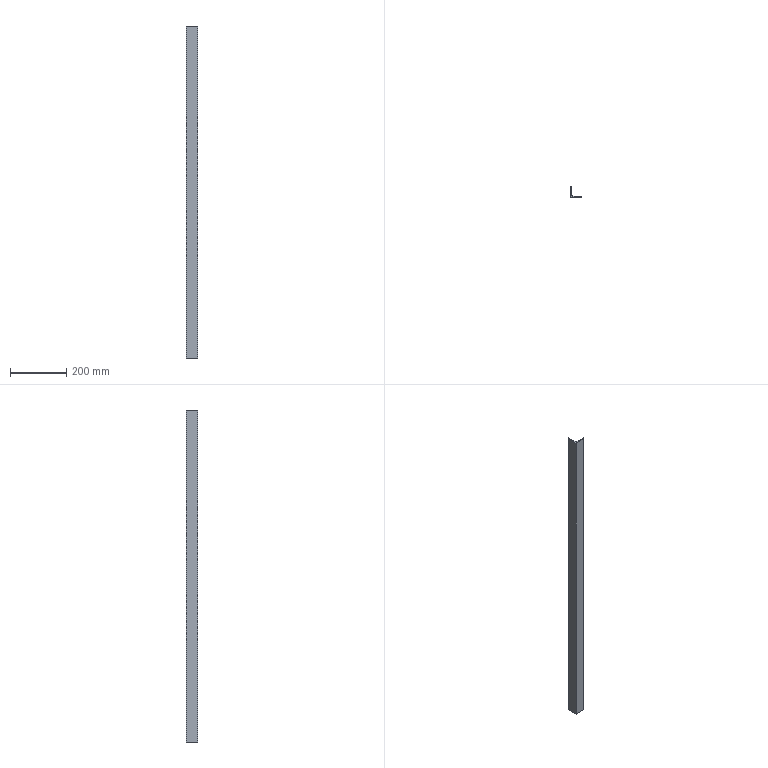Part | SolidWorks | features Extrusion 1 | 1 solid | 11 faces | box 40 x 40 x 1185 mm | volume 366598 mm3 | plane 8 | cylinder 3 | commonest cylinder face diameters 0.02 x2 10 x1
STEP:
#1=CARTESIAN_POINT('',(0.,0.,0.));
#2=VERTEX_POINT('',#1);
#3=CARTESIAN_POINT('',(40.,0.,0.));
#4=VERTEX_POINT('',#3);
#5=CARTESIAN_POINT('',(40.,0.,0.));
#6=DIRECTION('',(1.,0.,0.));
#7=VECTOR('',#6,1000.);
#8=LINE('',#5,#7);
#9=EDGE_CURVE('',#2,#4,#8,.T.);
#10=ORIENTED_EDGE('',*,*,#9,.T.);
#11=CARTESIAN_POINT('',(40.,0.,1185.));
#12=VERTEX_POINT('',#11);
#13=CARTESIAN_POINT('',(40.,0.,1185.));
#14=DIRECTION('',(0.,0.,-1.));
#15=VECTOR('',#14,1000.);
#16=LINE('',#13,#15);
#17=EDGE_CURVE('',#12,#4,#16,.T.);
#18=ORIENTED_EDGE('',*,*,#17,.F.);
#19=CARTESIAN_POINT('',(0.,0.,1185.));
#20=VERTEX_POINT('',#19);
#21=CARTESIAN_POINT('',(40.,0.,1185.));
#22=DIRECTION('',(1.,0.,0.));
#23=VECTOR('',#22,1000.);
#24=LINE('',#21,#23);
#25=EDGE_CURVE('',#20,#12,#24,.T.);
#26=ORIENTED_EDGE('',*,*,#25,.F.);
#27=CARTESIAN_POINT('',(0.,0.,1185.));
#28=DIRECTION('',(0.,0.,-1.));
#29=VECTOR('',#28,1000.);
#30=LINE('',#27,#29);
#31=EDGE_CURVE('',#20,#2,#30,.T.);
#32=ORIENTED_EDGE('',*,*,#31,.T.);
#33=EDGE_LOOP('',(#10,#18,#26,#32));
#34=FACE_OUTER_BOUND('',#33,.T.);
#35=CARTESIAN_POINT('',(40.,0.,1185.));
#36=DIRECTION('',(0.,1.,0.));
#37=DIRECTION('',(-1.,0.,0.));
#38=AXIS2_PLACEMENT_3D('',#35,#36,#37);
#39=PLANE('',#38);
#40=ADVANCED_FACE('',(#34),#39,.F.);
#41=CARTESIAN_POINT('',(40.,3.99,0.));
#42=VERTEX_POINT('',#41);
#43=CARTESIAN_POINT('',(40.,3.99,0.));
#44=DIRECTION('',(0.,1.,0.));
#45=VECTOR('',#44,1000.);
#46=LINE('',#43,#45);
#47=EDGE_CURVE('',#4,#42,#46,.T.);
#48=ORIENTED_EDGE('',*,*,#47,.T.);
#49=CARTESIAN_POINT('',(40.,3.99,1185.));
#50=VERTEX_POINT('',#49);
#51=CARTESIAN_POINT('',(40.,3.99,1185.));
#52=DIRECTION('',(0.,0.,-1.));
#53=VECTOR('',#52,1000.);
#54=LINE('',#51,#53);
#55=EDGE_CURVE('',#50,#42,#54,.T.);
#56=ORIENTED_EDGE('',*,*,#55,.F.);
#57=CARTESIAN_POINT('',(40.,3.99,1185.));
#58=DIRECTION('',(0.,1.,0.));
#59=VECTOR('',#58,1000.);
#60=LINE('',#57,#59);
#61=EDGE_CURVE('',#12,#50,#60,.T.);
#62=ORIENTED_EDGE('',*,*,#61,.F.);
#63=ORIENTED_EDGE('',*,*,#17,.T.);
#64=EDGE_LOOP('',(#48,#56,#62,#63));
#65=FACE_OUTER_BOUND('',#64,.T.);
#66=CARTESIAN_POINT('',(40.,3.99,1185.));
#67=DIRECTION('',(-1.,0.,0.));
#68=DIRECTION('',(0.,-1.,0.));
#69=AXIS2_PLACEMENT_3D('',#66,#67,#68);
#70=PLANE('',#69);
#71=ADVANCED_FACE('',(#65),#70,.F.);
#72=CARTESIAN_POINT('',(39.99,4.,0.));
#73=VERTEX_POINT('',#72);
#74=CARTESIAN_POINT('',(39.99,3.99,0.));
#75=DIRECTION('',(0.,0.,1.));
#76=DIRECTION('',(1.,0.,0.));
#77=AXIS2_PLACEMENT_3D('',#74,#75,#76);
#78=CIRCLE('',#77,0.01);
#79=EDGE_CURVE('',#42,#73,#78,.T.);
#80=ORIENTED_EDGE('',*,*,#79,.T.);
#81=CARTESIAN_POINT('',(39.99,4.,1185.));
#82=VERTEX_POINT('',#81);
#83=CARTESIAN_POINT('',(39.99,4.,1185.));
#84=DIRECTION('',(0.,0.,-1.));
#85=VECTOR('',#84,1000.);
#86=LINE('',#83,#85);
#87=EDGE_CURVE('',#82,#73,#86,.T.);
#88=ORIENTED_EDGE('',*,*,#87,.F.);
#89=CARTESIAN_POINT('',(39.99,3.99,1185.));
#90=DIRECTION('',(0.,0.,1.));
#91=DIRECTION('',(1.,0.,0.));
#92=AXIS2_PLACEMENT_3D('',#89,#90,#91);
#93=CIRCLE('',#92,0.01);
#94=EDGE_CURVE('',#50,#82,#93,.T.);
#95=ORIENTED_EDGE('',*,*,#94,.F.);
#96=ORIENTED_EDGE('',*,*,#55,.T.);
#97=EDGE_LOOP('',(#80,#88,#95,#96));
#98=FACE_OUTER_BOUND('',#97,.T.);
#99=CARTESIAN_POINT('',(39.99,3.99,1185.));
#100=DIRECTION('',(0.,0.,-1.));
#101=DIRECTION('',(-1.,0.,0.));
#102=AXIS2_PLACEMENT_3D('',#99,#100,#101);
#103=CYLINDRICAL_SURFACE('',#102,0.01);
#104=ADVANCED_FACE('',(#98),#103,.T.);
#105=CARTESIAN_POINT('',(9.,4.,0.));
#106=VERTEX_POINT('',#105);
#107=CARTESIAN_POINT('',(9.,4.,0.));
#108=DIRECTION('',(-1.,0.,0.));
#109=VECTOR('',#108,1000.);
#110=LINE('',#107,#109);
#111=EDGE_CURVE('',#73,#106,#110,.T.);
#112=ORIENTED_EDGE('',*,*,#111,.T.);
#113=CARTESIAN_POINT('',(9.,4.,1185.));
#114=VERTEX_POINT('',#113);
#115=CARTESIAN_POINT('',(9.,4.,1185.));
#116=DIRECTION('',(0.,0.,-1.));
#117=VECTOR('',#116,1000.);
#118=LINE('',#115,#117);
#119=EDGE_CURVE('',#114,#106,#118,.T.);
#120=ORIENTED_EDGE('',*,*,#119,.F.);
#121=CARTESIAN_POINT('',(9.,4.,1185.));
#122=DIRECTION('',(-1.,0.,0.));
#123=VECTOR('',#122,1000.);
#124=LINE('',#121,#123);
#125=EDGE_CURVE('',#82,#114,#124,.T.);
#126=ORIENTED_EDGE('',*,*,#125,.F.);
#127=ORIENTED_EDGE('',*,*,#87,.T.);
#128=EDGE_LOOP('',(#112,#120,#126,#127));
#129=FACE_OUTER_BOUND('',#128,.T.);
#130=CARTESIAN_POINT('',(9.,4.,1185.));
#131=DIRECTION('',(0.,-1.,0.));
#132=DIRECTION('',(1.,0.,0.));
#133=AXIS2_PLACEMENT_3D('',#130,#131,#132);
#134=PLANE('',#133);
#135=ADVANCED_FACE('',(#129),#134,.F.);
#136=CARTESIAN_POINT('',(4.,9.,0.));
#137=VERTEX_POINT('',#136);
#138=CARTESIAN_POINT('',(9.,9.,0.));
#139=DIRECTION('',(0.,0.,-1.));
#140=DIRECTION('',(-1.,0.,0.));
#141=AXIS2_PLACEMENT_3D('',#138,#139,#140);
#142=CIRCLE('',#141,5.);
#143=EDGE_CURVE('',#106,#137,#142,.T.);
#144=ORIENTED_EDGE('',*,*,#143,.T.);
#145=CARTESIAN_POINT('',(4.,9.,1185.));
#146=VERTEX_POINT('',#145);
#147=CARTESIAN_POINT('',(4.,9.,1185.));
#148=DIRECTION('',(0.,0.,-1.));
#149=VECTOR('',#148,1000.);
#150=LINE('',#147,#149);
#151=EDGE_CURVE('',#146,#137,#150,.T.);
#152=ORIENTED_EDGE('',*,*,#151,.F.);
#153=CARTESIAN_POINT('',(9.,9.,1185.));
#154=DIRECTION('',(0.,0.,-1.));
#155=DIRECTION('',(-1.,0.,0.));
#156=AXIS2_PLACEMENT_3D('',#153,#154,#155);
#157=CIRCLE('',#156,5.);
#158=EDGE_CURVE('',#114,#146,#157,.T.);
#159=ORIENTED_EDGE('',*,*,#158,.F.);
#160=ORIENTED_EDGE('',*,*,#119,.T.);
#161=EDGE_LOOP('',(#144,#152,#159,#160));
#162=FACE_OUTER_BOUND('',#161,.T.);
#163=CARTESIAN_POINT('',(9.,9.,1185.));
#164=DIRECTION('',(0.,0.,-1.));
#165=DIRECTION('',(-1.,0.,0.));
#166=AXIS2_PLACEMENT_3D('',#163,#164,#165);
#167=CYLINDRICAL_SURFACE('',#166,5.);
#168=ADVANCED_FACE('',(#162),#167,.F.);
#169=CARTESIAN_POINT('',(4.,39.99,0.));
#170=VERTEX_POINT('',#169);
#171=CARTESIAN_POINT('',(4.,39.99,0.));
#172=DIRECTION('',(0.,1.,0.));
#173=VECTOR('',#172,1000.);
#174=LINE('',#171,#173);
#175=EDGE_CURVE('',#137,#170,#174,.T.);
#176=ORIENTED_EDGE('',*,*,#175,.T.);
#177=CARTESIAN_POINT('',(4.,39.99,1185.));
#178=VERTEX_POINT('',#177);
#179=CARTESIAN_POINT('',(4.,39.99,1185.));
#180=DIRECTION('',(0.,0.,-1.));
#181=VECTOR('',#180,1000.);
#182=LINE('',#179,#181);
#183=EDGE_CURVE('',#178,#170,#182,.T.);
#184=ORIENTED_EDGE('',*,*,#183,.F.);
#185=CARTESIAN_POINT('',(4.,39.99,1185.));
#186=DIRECTION('',(0.,1.,0.));
#187=VECTOR('',#186,1000.);
#188=LINE('',#185,#187);
#189=EDGE_CURVE('',#146,#178,#188,.T.);
#190=ORIENTED_EDGE('',*,*,#189,.F.);
#191=ORIENTED_EDGE('',*,*,#151,.T.);
#192=EDGE_LOOP('',(#176,#184,#190,#191));
#193=FACE_OUTER_BOUND('',#192,.T.);
#194=CARTESIAN_POINT('',(4.,39.99,1185.));
#195=DIRECTION('',(-1.,0.,0.));
#196=DIRECTION('',(0.,-1.,0.));
#197=AXIS2_PLACEMENT_3D('',#194,#195,#196);
#198=PLANE('',#197);
#199=ADVANCED_FACE('',(#193),#198,.F.);
#200=CARTESIAN_POINT('',(3.99,40.,0.));
#201=VERTEX_POINT('',#200);
#202=CARTESIAN_POINT('',(3.99,39.99,0.));
#203=DIRECTION('',(0.,0.,1.));
#204=DIRECTION('',(1.,0.,0.));
#205=AXIS2_PLACEMENT_3D('',#202,#203,#204);
#206=CIRCLE('',#205,0.01);
#207=EDGE_CURVE('',#170,#201,#206,.T.);
#208=ORIENTED_EDGE('',*,*,#207,.T.);
#209=CARTESIAN_POINT('',(3.99,40.,1185.));
#210=VERTEX_POINT('',#209);
#211=CARTESIAN_POINT('',(3.99,40.,1185.));
#212=DIRECTION('',(0.,0.,-1.));
#213=VECTOR('',#212,1000.);
#214=LINE('',#211,#213);
#215=EDGE_CURVE('',#210,#201,#214,.T.);
#216=ORIENTED_EDGE('',*,*,#215,.F.);
#217=CARTESIAN_POINT('',(3.99,39.99,1185.));
#218=DIRECTION('',(0.,0.,1.));
#219=DIRECTION('',(1.,0.,0.));
#220=AXIS2_PLACEMENT_3D('',#217,#218,#219);
#221=CIRCLE('',#220,0.01);
#222=EDGE_CURVE('',#178,#210,#221,.T.);
#223=ORIENTED_EDGE('',*,*,#222,.F.);
#224=ORIENTED_EDGE('',*,*,#183,.T.);
#225=EDGE_LOOP('',(#208,#216,#223,#224));
#226=FACE_OUTER_BOUND('',#225,.T.);
#227=CARTESIAN_POINT('',(3.99,39.99,1185.));
#228=DIRECTION('',(0.,0.,-1.));
#229=DIRECTION('',(-1.,0.,0.));
#230=AXIS2_PLACEMENT_3D('',#227,#228,#229);
#231=CYLINDRICAL_SURFACE('',#230,0.01);
#232=ADVANCED_FACE('',(#226),#231,.T.);
#233=CARTESIAN_POINT('',(0.,40.,0.));
#234=VERTEX_POINT('',#233);
#235=CARTESIAN_POINT('',(0.,40.,0.));
#236=DIRECTION('',(-1.,0.,0.));
#237=VECTOR('',#236,1000.);
#238=LINE('',#235,#237);
#239=EDGE_CURVE('',#201,#234,#238,.T.);
#240=ORIENTED_EDGE('',*,*,#239,.T.);
#241=CARTESIAN_POINT('',(0.,40.,1185.));
#242=VERTEX_POINT('',#241);
#243=CARTESIAN_POINT('',(0.,40.,1185.));
#244=DIRECTION('',(0.,0.,-1.));
#245=VECTOR('',#244,1000.);
#246=LINE('',#243,#245);
#247=EDGE_CURVE('',#242,#234,#246,.T.);
#248=ORIENTED_EDGE('',*,*,#247,.F.);
#249=CARTESIAN_POINT('',(0.,40.,1185.));
#250=DIRECTION('',(-1.,0.,0.));
#251=VECTOR('',#250,1000.);
#252=LINE('',#249,#251);
#253=EDGE_CURVE('',#210,#242,#252,.T.);
#254=ORIENTED_EDGE('',*,*,#253,.F.);
#255=ORIENTED_EDGE('',*,*,#215,.T.);
#256=EDGE_LOOP('',(#240,#248,#254,#255));
#257=FACE_OUTER_BOUND('',#256,.T.);
#258=CARTESIAN_POINT('',(0.,40.,1185.));
#259=DIRECTION('',(0.,-1.,0.));
#260=DIRECTION('',(0.,0.,-1.));
#261=AXIS2_PLACEMENT_3D('',#258,#259,#260);
#262=PLANE('',#261);
#263=ADVANCED_FACE('',(#257),#262,.F.);
#264=CARTESIAN_POINT('',(0.,0.,0.));
#265=DIRECTION('',(0.,-1.,0.));
#266=VECTOR('',#265,1000.);
#267=LINE('',#264,#266);
#268=EDGE_CURVE('',#234,#2,#267,.T.);
#269=ORIENTED_EDGE('',*,*,#268,.T.);
#270=ORIENTED_EDGE('',*,*,#31,.F.);
#271=CARTESIAN_POINT('',(0.,0.,1185.));
#272=DIRECTION('',(0.,-1.,0.));
#273=VECTOR('',#272,1000.);
#274=LINE('',#271,#273);
#275=EDGE_CURVE('',#242,#20,#274,.T.);
#276=ORIENTED_EDGE('',*,*,#275,.F.);
#277=ORIENTED_EDGE('',*,*,#247,.T.);
#278=EDGE_LOOP('',(#269,#270,#276,#277));
#279=FACE_OUTER_BOUND('',#278,.T.);
#280=CARTESIAN_POINT('',(0.,0.,1185.));
#281=DIRECTION('',(1.,0.,0.));
#282=DIRECTION('',(0.,0.,-1.));
#283=AXIS2_PLACEMENT_3D('',#280,#281,#282);
#284=PLANE('',#283);
#285=ADVANCED_FACE('',(#279),#284,.F.);
#286=ORIENTED_EDGE('',*,*,#25,.T.);
#287=ORIENTED_EDGE('',*,*,#61,.T.);
#288=ORIENTED_EDGE('',*,*,#94,.T.);
#289=ORIENTED_EDGE('',*,*,#125,.T.);
#290=ORIENTED_EDGE('',*,*,#158,.T.);
#291=ORIENTED_EDGE('',*,*,#189,.T.);
#292=ORIENTED_EDGE('',*,*,#222,.T.);
#293=ORIENTED_EDGE('',*,*,#253,.T.);
#294=ORIENTED_EDGE('',*,*,#275,.T.);
#295=EDGE_LOOP('',(#286,#287,#288,#289,#290,#291,#292,#293,#294));
#296=FACE_OUTER_BOUND('',#295,.T.);
#297=CARTESIAN_POINT('',(3.99,39.99,1185.));
#298=DIRECTION('',(0.,0.,1.));
#299=DIRECTION('',(1.,0.,0.));
#300=AXIS2_PLACEMENT_3D('',#297,#298,#299);
#301=PLANE('',#300);
#302=ADVANCED_FACE('',(#296),#301,.T.);
#303=ORIENTED_EDGE('',*,*,#9,.F.);
#304=ORIENTED_EDGE('',*,*,#268,.F.);
#305=ORIENTED_EDGE('',*,*,#239,.F.);
#306=ORIENTED_EDGE('',*,*,#207,.F.);
#307=ORIENTED_EDGE('',*,*,#175,.F.);
#308=ORIENTED_EDGE('',*,*,#143,.F.);
#309=ORIENTED_EDGE('',*,*,#111,.F.);
#310=ORIENTED_EDGE('',*,*,#79,.F.);
#311=ORIENTED_EDGE('',*,*,#47,.F.);
#312=EDGE_LOOP('',(#303,#304,#305,#306,#307,#308,#309,#310,#311));
#313=FACE_OUTER_BOUND('',#312,.T.);
#314=CARTESIAN_POINT('',(3.99,39.99,0.));
#315=DIRECTION('',(0.,0.,1.));
#316=DIRECTION('',(1.,0.,0.));
#317=AXIS2_PLACEMENT_3D('',#314,#315,#316);
#318=PLANE('',#317);
#319=ADVANCED_FACE('',(#313),#318,.F.);
#320=CLOSED_SHELL('',(#40,#71,#104,#135,#168,#199,#232,#263,#285,#302,#319));
#321=MANIFOLD_SOLID_BREP('',#320);
#322=CARTESIAN_POINT('',(0.,0.,0.));
#323=DIRECTION('',(0.,0.,1.));
#324=DIRECTION('',(1.,0.,0.));
#325=AXIS2_PLACEMENT_3D('',#322,#323,#324);
#326=(LENGTH_UNIT()NAMED_UNIT(*)SI_UNIT(.MILLI.,.METRE.));
#327=UNCERTAINTY_MEASURE_WITH_UNIT(LENGTH_MEASURE(0.00001),#326,'','');
#328=(NAMED_UNIT(*)PLANE_ANGLE_UNIT()SI_UNIT($,.RADIAN.));
#329=(NAMED_UNIT(*)SI_UNIT($,.STERADIAN.)SOLID_ANGLE_UNIT());
#330=(GEOMETRIC_REPRESENTATION_CONTEXT(3)GLOBAL_UNCERTAINTY_ASSIGNED_CONTEXT((#327))GLOBAL_UNIT_ASSIGNED_CONTEXT((#326,#328,#329))REPRESENTATION_CONTEXT('',''));
#331=ADVANCED_BREP_SHAPE_REPRESENTATION('',(#321,#325),#330);